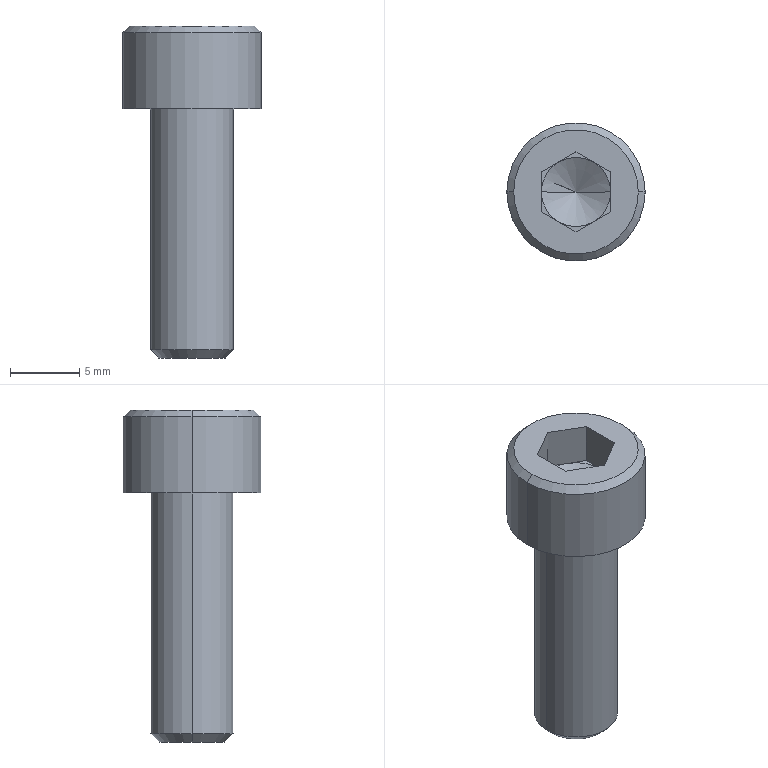Part | SolidWorks | features Chamfer 2, ICE 2, RevCut 1, Revolution 1 | 1 solid | 25 faces | box 10 x 10 x 24 mm | volume 898.677 mm3 | plane 15 | cone 6 | cylinder 4 | commonest cylinder face diameters 6 x2 10 x2
STEP:
#1=CARTESIAN_POINT('',(-2.387,0.,-18.));
#2=VERTEX_POINT('',#1);
#3=CARTESIAN_POINT('',(2.387,0.,-18.));
#4=VERTEX_POINT('',#3);
#5=CARTESIAN_POINT('',(0.,0.,-18.));
#6=DIRECTION('',(0.,0.,-1.));
#7=DIRECTION('',(-1.,0.,0.));
#8=AXIS2_PLACEMENT_3D('',#5,#6,#7);
#9=CIRCLE('',#8,2.387);
#10=EDGE_CURVE('',#2,#4,#9,.T.);
#11=ORIENTED_EDGE('',*,*,#10,.F.);
#12=CARTESIAN_POINT('',(-3.,0.,-17.387));
#13=VERTEX_POINT('',#12);
#14=CARTESIAN_POINT('',(-2.387,0.,-18.));
#15=DIRECTION('',(-0.7071,0.,0.7071));
#16=VECTOR('',#15,1000.);
#17=LINE('',#14,#16);
#18=EDGE_CURVE('',#2,#13,#17,.T.);
#19=ORIENTED_EDGE('',*,*,#18,.T.);
#20=CARTESIAN_POINT('',(3.,0.,-17.387));
#21=VERTEX_POINT('',#20);
#22=CARTESIAN_POINT('',(0.,0.,-17.387));
#23=DIRECTION('',(0.,0.,1.));
#24=DIRECTION('',(-1.,0.,0.));
#25=AXIS2_PLACEMENT_3D('',#22,#23,#24);
#26=CIRCLE('',#25,3.);
#27=EDGE_CURVE('',#21,#13,#26,.T.);
#28=ORIENTED_EDGE('',*,*,#27,.F.);
#29=CARTESIAN_POINT('',(2.387,0.,-18.));
#30=DIRECTION('',(0.7071,0.,0.7071));
#31=VECTOR('',#30,1000.);
#32=LINE('',#29,#31);
#33=EDGE_CURVE('',#4,#21,#32,.T.);
#34=ORIENTED_EDGE('',*,*,#33,.F.);
#35=EDGE_LOOP('',(#11,#19,#28,#34));
#36=FACE_OUTER_BOUND('',#35,.T.);
#37=CARTESIAN_POINT('',(0.,0.,-18.));
#38=DIRECTION('',(0.,0.,1.));
#39=DIRECTION('',(1.,0.,0.));
#40=AXIS2_PLACEMENT_3D('',#37,#38,#39);
#41=CONICAL_SURFACE('',#40,2.387,0.7854);
#42=ADVANCED_FACE('',(#36),#41,.T.);
#43=CARTESIAN_POINT('',(4.5,0.,6.));
#44=VERTEX_POINT('',#43);
#45=CARTESIAN_POINT('',(-4.5,0.,6.));
#46=VERTEX_POINT('',#45);
#47=CARTESIAN_POINT('',(0.,0.,6.));
#48=DIRECTION('',(0.,0.,1.));
#49=DIRECTION('',(1.,0.,0.));
#50=AXIS2_PLACEMENT_3D('',#47,#48,#49);
#51=CIRCLE('',#50,4.5);
#52=EDGE_CURVE('',#44,#46,#51,.T.);
#53=ORIENTED_EDGE('',*,*,#52,.F.);
#54=CARTESIAN_POINT('',(5.,0.,5.5));
#55=VERTEX_POINT('',#54);
#56=CARTESIAN_POINT('',(4.5,0.,6.));
#57=DIRECTION('',(0.7071,0.,-0.7071));
#58=VECTOR('',#57,1000.);
#59=LINE('',#56,#58);
#60=EDGE_CURVE('',#44,#55,#59,.T.);
#61=ORIENTED_EDGE('',*,*,#60,.T.);
#62=CARTESIAN_POINT('',(-5.,0.,5.5));
#63=VERTEX_POINT('',#62);
#64=CARTESIAN_POINT('',(0.,0.,5.5));
#65=DIRECTION('',(0.,0.,-1.));
#66=DIRECTION('',(1.,0.,0.));
#67=AXIS2_PLACEMENT_3D('',#64,#65,#66);
#68=CIRCLE('',#67,5.);
#69=EDGE_CURVE('',#63,#55,#68,.T.);
#70=ORIENTED_EDGE('',*,*,#69,.F.);
#71=CARTESIAN_POINT('',(-4.5,0.,6.));
#72=DIRECTION('',(-0.7071,0.,-0.7071));
#73=VECTOR('',#72,1000.);
#74=LINE('',#71,#73);
#75=EDGE_CURVE('',#46,#63,#74,.T.);
#76=ORIENTED_EDGE('',*,*,#75,.F.);
#77=EDGE_LOOP('',(#53,#61,#70,#76));
#78=FACE_OUTER_BOUND('',#77,.T.);
#79=CARTESIAN_POINT('',(0.,0.,6.));
#80=DIRECTION('',(0.,0.,-1.));
#81=DIRECTION('',(-1.,0.,0.));
#82=AXIS2_PLACEMENT_3D('',#79,#80,#81);
#83=CONICAL_SURFACE('',#82,4.5,0.7854);
#84=ADVANCED_FACE('',(#78),#83,.T.);
#85=CARTESIAN_POINT('',(0.,0.,1.557));
#86=VERTEX_POINT('',#85);
#87=CARTESIAN_POINT('',(2.5,0.,3.));
#88=VERTEX_POINT('',#87);
#89=CARTESIAN_POINT('',(0.,0.,1.557));
#90=DIRECTION('',(0.866,0.,0.5));
#91=VECTOR('',#90,1000.);
#92=LINE('',#89,#91);
#93=EDGE_CURVE('',#86,#88,#92,.T.);
#94=ORIENTED_EDGE('',*,*,#93,.F.);
#95=CARTESIAN_POINT('',(-2.5,0.,3.));
#96=VERTEX_POINT('',#95);
#97=CARTESIAN_POINT('',(0.,0.,1.557));
#98=DIRECTION('',(-0.866,0.,0.5));
#99=VECTOR('',#98,1000.);
#100=LINE('',#97,#99);
#101=EDGE_CURVE('',#86,#96,#100,.T.);
#102=ORIENTED_EDGE('',*,*,#101,.T.);
#103=CARTESIAN_POINT('',(-1.25,-2.165,3.));
#104=VERTEX_POINT('',#103);
#105=CARTESIAN_POINT('',(0.,0.,3.));
#106=DIRECTION('',(0.,0.,-1.));
#107=DIRECTION('',(-1.,0.,0.));
#108=AXIS2_PLACEMENT_3D('',#105,#106,#107);
#109=CIRCLE('',#108,2.5);
#110=EDGE_CURVE('',#104,#96,#109,.T.);
#111=ORIENTED_EDGE('',*,*,#110,.F.);
#112=CARTESIAN_POINT('',(1.25,-2.165,3.));
#113=VERTEX_POINT('',#112);
#114=CARTESIAN_POINT('',(0.,0.,3.));
#115=DIRECTION('',(0.,0.,-1.));
#116=DIRECTION('',(-1.,0.,0.));
#117=AXIS2_PLACEMENT_3D('',#114,#115,#116);
#118=CIRCLE('',#117,2.5);
#119=EDGE_CURVE('',#113,#104,#118,.T.);
#120=ORIENTED_EDGE('',*,*,#119,.F.);
#121=CARTESIAN_POINT('',(0.,0.,3.));
#122=DIRECTION('',(0.,0.,-1.));
#123=DIRECTION('',(-1.,0.,0.));
#124=AXIS2_PLACEMENT_3D('',#121,#122,#123);
#125=CIRCLE('',#124,2.5);
#126=EDGE_CURVE('',#88,#113,#125,.T.);
#127=ORIENTED_EDGE('',*,*,#126,.F.);
#128=EDGE_LOOP('',(#94,#102,#111,#120,#127));
#129=FACE_OUTER_BOUND('',#128,.T.);
#130=CARTESIAN_POINT('',(0.,0.,1001.557));
#131=DIRECTION('',(0.,0.,1.));
#132=DIRECTION('',(1.,0.,0.));
#133=AXIS2_PLACEMENT_3D('',#130,#131,#132);
#134=CONICAL_SURFACE('',#133,1732.051,1.047);
#135=ADVANCED_FACE('',(#129),#134,.F.);
#136=ORIENTED_EDGE('',*,*,#27,.T.);
#137=CARTESIAN_POINT('',(-3.,0.,0.));
#138=VERTEX_POINT('',#137);
#139=CARTESIAN_POINT('',(-3.,0.,-18.));
#140=DIRECTION('',(0.,0.,1.));
#141=VECTOR('',#140,1000.);
#142=LINE('',#139,#141);
#143=EDGE_CURVE('',#13,#138,#142,.T.);
#144=ORIENTED_EDGE('',*,*,#143,.T.);
#145=CARTESIAN_POINT('',(3.,0.,0.));
#146=VERTEX_POINT('',#145);
#147=CARTESIAN_POINT('',(0.,0.,0.));
#148=DIRECTION('',(0.,0.,-1.));
#149=DIRECTION('',(-1.,0.,0.));
#150=AXIS2_PLACEMENT_3D('',#147,#148,#149);
#151=CIRCLE('',#150,3.);
#152=EDGE_CURVE('',#138,#146,#151,.T.);
#153=ORIENTED_EDGE('',*,*,#152,.T.);
#154=CARTESIAN_POINT('',(3.,0.,-18.));
#155=DIRECTION('',(0.,0.,1.));
#156=VECTOR('',#155,1000.);
#157=LINE('',#154,#156);
#158=EDGE_CURVE('',#21,#146,#157,.T.);
#159=ORIENTED_EDGE('',*,*,#158,.F.);
#160=EDGE_LOOP('',(#136,#144,#153,#159));
#161=FACE_OUTER_BOUND('',#160,.T.);
#162=CARTESIAN_POINT('',(0.,0.,-18.));
#163=DIRECTION('',(0.,0.,1.));
#164=DIRECTION('',(1.,0.,0.));
#165=AXIS2_PLACEMENT_3D('',#162,#163,#164);
#166=CYLINDRICAL_SURFACE('',#165,3.);
#167=ADVANCED_FACE('',(#161),#166,.T.);
#168=CARTESIAN_POINT('',(5.,0.,0.));
#169=VERTEX_POINT('',#168);
#170=CARTESIAN_POINT('',(-5.,0.,0.));
#171=VERTEX_POINT('',#170);
#172=CARTESIAN_POINT('',(0.,0.,0.));
#173=DIRECTION('',(0.,0.,1.));
#174=DIRECTION('',(1.,0.,0.));
#175=AXIS2_PLACEMENT_3D('',#172,#173,#174);
#176=CIRCLE('',#175,5.);
#177=EDGE_CURVE('',#169,#171,#176,.T.);
#178=ORIENTED_EDGE('',*,*,#177,.T.);
#179=CARTESIAN_POINT('',(-5.,0.,0.));
#180=DIRECTION('',(0.,0.,1.));
#181=VECTOR('',#180,1000.);
#182=LINE('',#179,#181);
#183=EDGE_CURVE('',#171,#63,#182,.T.);
#184=ORIENTED_EDGE('',*,*,#183,.T.);
#185=ORIENTED_EDGE('',*,*,#69,.T.);
#186=CARTESIAN_POINT('',(5.,0.,0.));
#187=DIRECTION('',(0.,0.,1.));
#188=VECTOR('',#187,1000.);
#189=LINE('',#186,#188);
#190=EDGE_CURVE('',#169,#55,#189,.T.);
#191=ORIENTED_EDGE('',*,*,#190,.F.);
#192=EDGE_LOOP('',(#178,#184,#185,#191));
#193=FACE_OUTER_BOUND('',#192,.T.);
#194=CARTESIAN_POINT('',(0.,0.,0.));
#195=DIRECTION('',(0.,0.,1.));
#196=DIRECTION('',(1.,0.,0.));
#197=AXIS2_PLACEMENT_3D('',#194,#195,#196);
#198=CYLINDRICAL_SURFACE('',#197,5.);
#199=ADVANCED_FACE('',(#193),#198,.T.);
#200=CARTESIAN_POINT('',(-2.5,1.443,3.));
#201=VERTEX_POINT('',#200);
#202=CARTESIAN_POINT('',(-2.5,1.443,3.));
#203=DIRECTION('',(0.,-1.,0.));
#204=VECTOR('',#203,1000.);
#205=LINE('',#202,#204);
#206=EDGE_CURVE('',#201,#96,#205,.T.);
#207=ORIENTED_EDGE('',*,*,#206,.T.);
#208=CARTESIAN_POINT('',(-1.25,2.165,3.));
#209=VERTEX_POINT('',#208);
#210=CARTESIAN_POINT('',(0.,0.,3.));
#211=DIRECTION('',(0.,0.,-1.));
#212=DIRECTION('',(-1.,0.,0.));
#213=AXIS2_PLACEMENT_3D('',#210,#211,#212);
#214=CIRCLE('',#213,2.5);
#215=EDGE_CURVE('',#96,#209,#214,.T.);
#216=ORIENTED_EDGE('',*,*,#215,.T.);
#217=CARTESIAN_POINT('',(0.,2.887,3.));
#218=DIRECTION('',(-0.866,-0.5,0.));
#219=VECTOR('',#218,1000.);
#220=LINE('',#217,#219);
#221=EDGE_CURVE('',#209,#201,#220,.T.);
#222=ORIENTED_EDGE('',*,*,#221,.T.);
#223=EDGE_LOOP('',(#207,#216,#222));
#224=FACE_OUTER_BOUND('',#223,.T.);
#225=CARTESIAN_POINT('',(0.,0.,3.));
#226=DIRECTION('',(0.,0.,1.));
#227=DIRECTION('',(1.,0.,0.));
#228=AXIS2_PLACEMENT_3D('',#225,#226,#227);
#229=PLANE('',#228);
#230=ADVANCED_FACE('',(#224),#229,.T.);
#231=CARTESIAN_POINT('',(0.,2.887,3.));
#232=VERTEX_POINT('',#231);
#233=CARTESIAN_POINT('',(0.,2.887,3.));
#234=DIRECTION('',(-0.866,-0.5,0.));
#235=VECTOR('',#234,1000.);
#236=LINE('',#233,#235);
#237=EDGE_CURVE('',#232,#209,#236,.T.);
#238=ORIENTED_EDGE('',*,*,#237,.T.);
#239=CARTESIAN_POINT('',(1.25,2.165,3.));
#240=VERTEX_POINT('',#239);
#241=CARTESIAN_POINT('',(0.,0.,3.));
#242=DIRECTION('',(0.,0.,-1.));
#243=DIRECTION('',(-1.,0.,0.));
#244=AXIS2_PLACEMENT_3D('',#241,#242,#243);
#245=CIRCLE('',#244,2.5);
#246=EDGE_CURVE('',#209,#240,#245,.T.);
#247=ORIENTED_EDGE('',*,*,#246,.T.);
#248=CARTESIAN_POINT('',(2.5,1.443,3.));
#249=DIRECTION('',(-0.866,0.5,0.));
#250=VECTOR('',#249,1000.);
#251=LINE('',#248,#250);
#252=EDGE_CURVE('',#240,#232,#251,.T.);
#253=ORIENTED_EDGE('',*,*,#252,.T.);
#254=EDGE_LOOP('',(#238,#247,#253));
#255=FACE_OUTER_BOUND('',#254,.T.);
#256=CARTESIAN_POINT('',(0.,0.,3.));
#257=DIRECTION('',(0.,0.,1.));
#258=DIRECTION('',(1.,0.,0.));
#259=AXIS2_PLACEMENT_3D('',#256,#257,#258);
#260=PLANE('',#259);
#261=ADVANCED_FACE('',(#255),#260,.T.);
#262=CARTESIAN_POINT('',(2.5,1.443,3.));
#263=VERTEX_POINT('',#262);
#264=CARTESIAN_POINT('',(2.5,1.443,3.));
#265=DIRECTION('',(-0.866,0.5,0.));
#266=VECTOR('',#265,1000.);
#267=LINE('',#264,#266);
#268=EDGE_CURVE('',#263,#240,#267,.T.);
#269=ORIENTED_EDGE('',*,*,#268,.T.);
#270=CARTESIAN_POINT('',(0.,0.,3.));
#271=DIRECTION('',(0.,0.,-1.));
#272=DIRECTION('',(-1.,0.,0.));
#273=AXIS2_PLACEMENT_3D('',#270,#271,#272);
#274=CIRCLE('',#273,2.5);
#275=EDGE_CURVE('',#240,#88,#274,.T.);
#276=ORIENTED_EDGE('',*,*,#275,.T.);
#277=CARTESIAN_POINT('',(2.5,-1.443,3.));
#278=DIRECTION('',(0.,1.,0.));
#279=VECTOR('',#278,1000.);
#280=LINE('',#277,#279);
#281=EDGE_CURVE('',#88,#263,#280,.T.);
#282=ORIENTED_EDGE('',*,*,#281,.T.);
#283=EDGE_LOOP('',(#269,#276,#282));
#284=FACE_OUTER_BOUND('',#283,.T.);
#285=CARTESIAN_POINT('',(0.,0.,3.));
#286=DIRECTION('',(0.,0.,1.));
#287=DIRECTION('',(1.,0.,0.));
#288=AXIS2_PLACEMENT_3D('',#285,#286,#287);
#289=PLANE('',#288);
#290=ADVANCED_FACE('',(#284),#289,.T.);
#291=CARTESIAN_POINT('',(2.5,-1.443,3.));
#292=VERTEX_POINT('',#291);
#293=CARTESIAN_POINT('',(2.5,-1.443,3.));
#294=DIRECTION('',(0.,1.,0.));
#295=VECTOR('',#294,1000.);
#296=LINE('',#293,#295);
#297=EDGE_CURVE('',#292,#88,#296,.T.);
#298=ORIENTED_EDGE('',*,*,#297,.T.);
#299=ORIENTED_EDGE('',*,*,#126,.T.);
#300=CARTESIAN_POINT('',(0.,-2.887,3.));
#301=DIRECTION('',(0.866,0.5,0.));
#302=VECTOR('',#301,1000.);
#303=LINE('',#300,#302);
#304=EDGE_CURVE('',#113,#292,#303,.T.);
#305=ORIENTED_EDGE('',*,*,#304,.T.);
#306=EDGE_LOOP('',(#298,#299,#305));
#307=FACE_OUTER_BOUND('',#306,.T.);
#308=CARTESIAN_POINT('',(0.,0.,3.));
#309=DIRECTION('',(0.,0.,1.));
#310=DIRECTION('',(1.,0.,0.));
#311=AXIS2_PLACEMENT_3D('',#308,#309,#310);
#312=PLANE('',#311);
#313=ADVANCED_FACE('',(#307),#312,.T.);
#314=CARTESIAN_POINT('',(0.,-2.887,3.));
#315=VERTEX_POINT('',#314);
#316=CARTESIAN_POINT('',(0.,-2.887,3.));
#317=DIRECTION('',(0.866,0.5,0.));
#318=VECTOR('',#317,1000.);
#319=LINE('',#316,#318);
#320=EDGE_CURVE('',#315,#113,#319,.T.);
#321=ORIENTED_EDGE('',*,*,#320,.T.);
#322=ORIENTED_EDGE('',*,*,#119,.T.);
#323=CARTESIAN_POINT('',(-2.5,-1.443,3.));
#324=DIRECTION('',(0.866,-0.5,0.));
#325=VECTOR('',#324,1000.);
#326=LINE('',#323,#325);
#327=EDGE_CURVE('',#104,#315,#326,.T.);
#328=ORIENTED_EDGE('',*,*,#327,.T.);
#329=EDGE_LOOP('',(#321,#322,#328));
#330=FACE_OUTER_BOUND('',#329,.T.);
#331=CARTESIAN_POINT('',(0.,0.,3.));
#332=DIRECTION('',(0.,0.,1.));
#333=DIRECTION('',(1.,0.,0.));
#334=AXIS2_PLACEMENT_3D('',#331,#332,#333);
#335=PLANE('',#334);
#336=ADVANCED_FACE('',(#330),#335,.T.);
#337=CARTESIAN_POINT('',(-2.5,-1.443,3.));
#338=VERTEX_POINT('',#337);
#339=CARTESIAN_POINT('',(-2.5,-1.443,3.));
#340=DIRECTION('',(0.866,-0.5,0.));
#341=VECTOR('',#340,1000.);
#342=LINE('',#339,#341);
#343=EDGE_CURVE('',#338,#104,#342,.T.);
#344=ORIENTED_EDGE('',*,*,#343,.T.);
#345=ORIENTED_EDGE('',*,*,#110,.T.);
#346=CARTESIAN_POINT('',(-2.5,1.443,3.));
#347=DIRECTION('',(0.,-1.,0.));
#348=VECTOR('',#347,1000.);
#349=LINE('',#346,#348);
#350=EDGE_CURVE('',#96,#338,#349,.T.);
#351=ORIENTED_EDGE('',*,*,#350,.T.);
#352=EDGE_LOOP('',(#344,#345,#351));
#353=FACE_OUTER_BOUND('',#352,.T.);
#354=CARTESIAN_POINT('',(0.,0.,3.));
#355=DIRECTION('',(0.,0.,1.));
#356=DIRECTION('',(1.,0.,0.));
#357=AXIS2_PLACEMENT_3D('',#354,#355,#356);
#358=PLANE('',#357);
#359=ADVANCED_FACE('',(#353),#358,.T.);
#360=ORIENTED_EDGE('',*,*,#177,.F.);
#361=CARTESIAN_POINT('',(0.,0.,0.));
#362=DIRECTION('',(0.,0.,1.));
#363=DIRECTION('',(1.,0.,0.));
#364=AXIS2_PLACEMENT_3D('',#361,#362,#363);
#365=CIRCLE('',#364,5.);
#366=EDGE_CURVE('',#171,#169,#365,.T.);
#367=ORIENTED_EDGE('',*,*,#366,.F.);
#368=EDGE_LOOP('',(#360,#367));
#369=FACE_OUTER_BOUND('',#368,.T.);
#370=CARTESIAN_POINT('',(0.,0.,0.));
#371=DIRECTION('',(0.,0.,-1.));
#372=DIRECTION('',(-1.,0.,0.));
#373=AXIS2_PLACEMENT_3D('',#370,#371,#372);
#374=CIRCLE('',#373,3.);
#375=EDGE_CURVE('',#146,#138,#374,.T.);
#376=ORIENTED_EDGE('',*,*,#375,.F.);
#377=ORIENTED_EDGE('',*,*,#152,.F.);
#378=EDGE_LOOP('',(#376,#377));
#379=FACE_BOUND('',#378,.T.);
#380=CARTESIAN_POINT('',(5.,0.,0.));
#381=DIRECTION('',(0.,0.,-1.));
#382=DIRECTION('',(-1.,0.,0.));
#383=AXIS2_PLACEMENT_3D('',#380,#381,#382);
#384=PLANE('',#383);
#385=ADVANCED_FACE('',(#369,#379),#384,.T.);
#386=ORIENTED_EDGE('',*,*,#183,.F.);
#387=ORIENTED_EDGE('',*,*,#366,.T.);
#388=ORIENTED_EDGE('',*,*,#190,.T.);
#389=CARTESIAN_POINT('',(0.,0.,5.5));
#390=DIRECTION('',(0.,0.,-1.));
#391=DIRECTION('',(1.,0.,0.));
#392=AXIS2_PLACEMENT_3D('',#389,#390,#391);
#393=CIRCLE('',#392,5.);
#394=EDGE_CURVE('',#55,#63,#393,.T.);
#395=ORIENTED_EDGE('',*,*,#394,.T.);
#396=EDGE_LOOP('',(#386,#387,#388,#395));
#397=FACE_OUTER_BOUND('',#396,.T.);
#398=CARTESIAN_POINT('',(0.,0.,0.));
#399=DIRECTION('',(0.,0.,1.));
#400=DIRECTION('',(1.,0.,0.));
#401=AXIS2_PLACEMENT_3D('',#398,#399,#400);
#402=CYLINDRICAL_SURFACE('',#401,5.);
#403=ADVANCED_FACE('',(#397),#402,.T.);
#404=CARTESIAN_POINT('',(0.,0.,6.));
#405=DIRECTION('',(0.,0.,1.));
#406=DIRECTION('',(1.,0.,0.));
#407=AXIS2_PLACEMENT_3D('',#404,#405,#406);
#408=CIRCLE('',#407,4.5);
#409=EDGE_CURVE('',#46,#44,#408,.T.);
#410=ORIENTED_EDGE('',*,*,#409,.T.);
#411=ORIENTED_EDGE('',*,*,#52,.T.);
#412=EDGE_LOOP('',(#410,#411));
#413=FACE_OUTER_BOUND('',#412,.T.);
#414=CARTESIAN_POINT('',(2.5,-1.443,6.));
#415=VERTEX_POINT('',#414);
#416=CARTESIAN_POINT('',(2.5,1.443,6.));
#417=VERTEX_POINT('',#416);
#418=CARTESIAN_POINT('',(2.5,-1.443,6.));
#419=DIRECTION('',(0.,1.,0.));
#420=VECTOR('',#419,1000.);
#421=LINE('',#418,#420);
#422=EDGE_CURVE('',#415,#417,#421,.T.);
#423=ORIENTED_EDGE('',*,*,#422,.F.);
#424=CARTESIAN_POINT('',(0.,-2.887,6.));
#425=VERTEX_POINT('',#424);
#426=CARTESIAN_POINT('',(0.,-2.887,6.));
#427=DIRECTION('',(0.866,0.5,0.));
#428=VECTOR('',#427,1000.);
#429=LINE('',#426,#428);
#430=EDGE_CURVE('',#425,#415,#429,.T.);
#431=ORIENTED_EDGE('',*,*,#430,.F.);
#432=CARTESIAN_POINT('',(-2.5,-1.443,6.));
#433=VERTEX_POINT('',#432);
#434=CARTESIAN_POINT('',(-2.5,-1.443,6.));
#435=DIRECTION('',(0.866,-0.5,0.));
#436=VECTOR('',#435,1000.);
#437=LINE('',#434,#436);
#438=EDGE_CURVE('',#433,#425,#437,.T.);
#439=ORIENTED_EDGE('',*,*,#438,.F.);
#440=CARTESIAN_POINT('',(-2.5,1.443,6.));
#441=VERTEX_POINT('',#440);
#442=CARTESIAN_POINT('',(-2.5,1.443,6.));
#443=DIRECTION('',(0.,-1.,0.));
#444=VECTOR('',#443,1000.);
#445=LINE('',#442,#444);
#446=EDGE_CURVE('',#441,#433,#445,.T.);
#447=ORIENTED_EDGE('',*,*,#446,.F.);
#448=CARTESIAN_POINT('',(0.,2.887,6.));
#449=VERTEX_POINT('',#448);
#450=CARTESIAN_POINT('',(0.,2.887,6.));
#451=DIRECTION('',(-0.866,-0.5,0.));
#452=VECTOR('',#451,1000.);
#453=LINE('',#450,#452);
#454=EDGE_CURVE('',#449,#441,#453,.T.);
#455=ORIENTED_EDGE('',*,*,#454,.F.);
#456=CARTESIAN_POINT('',(2.5,1.443,6.));
#457=DIRECTION('',(-0.866,0.5,0.));
#458=VECTOR('',#457,1000.);
#459=LINE('',#456,#458);
#460=EDGE_CURVE('',#417,#449,#459,.T.);
#461=ORIENTED_EDGE('',*,*,#460,.F.);
#462=EDGE_LOOP('',(#423,#431,#439,#447,#455,#461));
#463=FACE_BOUND('',#462,.T.);
#464=CARTESIAN_POINT('',(0.,0.,6.));
#465=DIRECTION('',(0.,0.,1.));
#466=DIRECTION('',(1.,0.,0.));
#467=AXIS2_PLACEMENT_3D('',#464,#465,#466);
#468=PLANE('',#467);
#469=ADVANCED_FACE('',(#413,#463),#468,.T.);
#470=ORIENTED_EDGE('',*,*,#143,.F.);
#471=CARTESIAN_POINT('',(0.,0.,-17.387));
#472=DIRECTION('',(0.,0.,1.));
#473=DIRECTION('',(-1.,0.,0.));
#474=AXIS2_PLACEMENT_3D('',#471,#472,#473);
#475=CIRCLE('',#474,3.);
#476=EDGE_CURVE('',#13,#21,#475,.T.);
#477=ORIENTED_EDGE('',*,*,#476,.T.);
#478=ORIENTED_EDGE('',*,*,#158,.T.);
#479=ORIENTED_EDGE('',*,*,#375,.T.);
#480=EDGE_LOOP('',(#470,#477,#478,#479));
#481=FACE_OUTER_BOUND('',#480,.T.);
#482=CARTESIAN_POINT('',(0.,0.,-18.));
#483=DIRECTION('',(0.,0.,1.));
#484=DIRECTION('',(1.,0.,0.));
#485=AXIS2_PLACEMENT_3D('',#482,#483,#484);
#486=CYLINDRICAL_SURFACE('',#485,3.);
#487=ADVANCED_FACE('',(#481),#486,.T.);
#488=CARTESIAN_POINT('',(0.,0.,-18.));
#489=DIRECTION('',(0.,0.,-1.));
#490=DIRECTION('',(-1.,0.,0.));
#491=AXIS2_PLACEMENT_3D('',#488,#489,#490);
#492=CIRCLE('',#491,2.387);
#493=EDGE_CURVE('',#4,#2,#492,.T.);
#494=ORIENTED_EDGE('',*,*,#493,.T.);
#495=ORIENTED_EDGE('',*,*,#10,.T.);
#496=EDGE_LOOP('',(#494,#495));
#497=FACE_OUTER_BOUND('',#496,.T.);
#498=CARTESIAN_POINT('',(0.,0.,-18.));
#499=DIRECTION('',(0.,0.,-1.));
#500=DIRECTION('',(-1.,0.,0.));
#501=AXIS2_PLACEMENT_3D('',#498,#499,#500);
#502=PLANE('',#501);
#503=ADVANCED_FACE('',(#497),#502,.T.);
#504=ORIENTED_EDGE('',*,*,#422,.T.);
#505=CARTESIAN_POINT('',(2.5,1.443,3.));
#506=DIRECTION('',(0.,0.,1.));
#507=VECTOR('',#506,1000.);
#508=LINE('',#505,#507);
#509=EDGE_CURVE('',#263,#417,#508,.T.);
#510=ORIENTED_EDGE('',*,*,#509,.F.);
#511=ORIENTED_EDGE('',*,*,#281,.F.);
#512=ORIENTED_EDGE('',*,*,#297,.F.);
#513=CARTESIAN_POINT('',(2.5,-1.443,3.));
#514=DIRECTION('',(0.,0.,1.));
#515=VECTOR('',#514,1000.);
#516=LINE('',#513,#515);
#517=EDGE_CURVE('',#292,#415,#516,.T.);
#518=ORIENTED_EDGE('',*,*,#517,.T.);
#519=EDGE_LOOP('',(#504,#510,#511,#512,#518));
#520=FACE_OUTER_BOUND('',#519,.T.);
#521=CARTESIAN_POINT('',(2.5,-1.443,3.));
#522=DIRECTION('',(1.,0.,0.));
#523=DIRECTION('',(0.,1.,0.));
#524=AXIS2_PLACEMENT_3D('',#521,#522,#523);
#525=PLANE('',#524);
#526=ADVANCED_FACE('',(#520),#525,.F.);
#527=ORIENTED_EDGE('',*,*,#430,.T.);
#528=ORIENTED_EDGE('',*,*,#517,.F.);
#529=ORIENTED_EDGE('',*,*,#304,.F.);
#530=ORIENTED_EDGE('',*,*,#320,.F.);
#531=CARTESIAN_POINT('',(0.,-2.887,3.));
#532=DIRECTION('',(0.,0.,1.));
#533=VECTOR('',#532,1000.);
#534=LINE('',#531,#533);
#535=EDGE_CURVE('',#315,#425,#534,.T.);
#536=ORIENTED_EDGE('',*,*,#535,.T.);
#537=EDGE_LOOP('',(#527,#528,#529,#530,#536));
#538=FACE_OUTER_BOUND('',#537,.T.);
#539=CARTESIAN_POINT('',(0.,-2.887,3.));
#540=DIRECTION('',(0.5,-0.866,0.));
#541=DIRECTION('',(0.866,0.5,0.));
#542=AXIS2_PLACEMENT_3D('',#539,#540,#541);
#543=PLANE('',#542);
#544=ADVANCED_FACE('',(#538),#543,.F.);
#545=ORIENTED_EDGE('',*,*,#438,.T.);
#546=ORIENTED_EDGE('',*,*,#535,.F.);
#547=ORIENTED_EDGE('',*,*,#327,.F.);
#548=ORIENTED_EDGE('',*,*,#343,.F.);
#549=CARTESIAN_POINT('',(-2.5,-1.443,3.));
#550=DIRECTION('',(0.,0.,1.));
#551=VECTOR('',#550,1000.);
#552=LINE('',#549,#551);
#553=EDGE_CURVE('',#338,#433,#552,.T.);
#554=ORIENTED_EDGE('',*,*,#553,.T.);
#555=EDGE_LOOP('',(#545,#546,#547,#548,#554));
#556=FACE_OUTER_BOUND('',#555,.T.);
#557=CARTESIAN_POINT('',(-2.5,-1.443,3.));
#558=DIRECTION('',(-0.5,-0.866,0.));
#559=DIRECTION('',(0.866,-0.5,0.));
#560=AXIS2_PLACEMENT_3D('',#557,#558,#559);
#561=PLANE('',#560);
#562=ADVANCED_FACE('',(#556),#561,.F.);
#563=ORIENTED_EDGE('',*,*,#446,.T.);
#564=ORIENTED_EDGE('',*,*,#553,.F.);
#565=ORIENTED_EDGE('',*,*,#350,.F.);
#566=ORIENTED_EDGE('',*,*,#206,.F.);
#567=CARTESIAN_POINT('',(-2.5,1.443,3.));
#568=DIRECTION('',(0.,0.,1.));
#569=VECTOR('',#568,1000.);
#570=LINE('',#567,#569);
#571=EDGE_CURVE('',#201,#441,#570,.T.);
#572=ORIENTED_EDGE('',*,*,#571,.T.);
#573=EDGE_LOOP('',(#563,#564,#565,#566,#572));
#574=FACE_OUTER_BOUND('',#573,.T.);
#575=CARTESIAN_POINT('',(-2.5,1.443,3.));
#576=DIRECTION('',(-1.,0.,0.));
#577=DIRECTION('',(0.,-1.,0.));
#578=AXIS2_PLACEMENT_3D('',#575,#576,#577);
#579=PLANE('',#578);
#580=ADVANCED_FACE('',(#574),#579,.F.);
#581=ORIENTED_EDGE('',*,*,#454,.T.);
#582=ORIENTED_EDGE('',*,*,#571,.F.);
#583=ORIENTED_EDGE('',*,*,#221,.F.);
#584=ORIENTED_EDGE('',*,*,#237,.F.);
#585=CARTESIAN_POINT('',(0.,2.887,3.));
#586=DIRECTION('',(0.,0.,1.));
#587=VECTOR('',#586,1000.);
#588=LINE('',#585,#587);
#589=EDGE_CURVE('',#232,#449,#588,.T.);
#590=ORIENTED_EDGE('',*,*,#589,.T.);
#591=EDGE_LOOP('',(#581,#582,#583,#584,#590));
#592=FACE_OUTER_BOUND('',#591,.T.);
#593=CARTESIAN_POINT('',(0.,2.887,3.));
#594=DIRECTION('',(-0.5,0.866,0.));
#595=DIRECTION('',(-0.866,-0.5,0.));
#596=AXIS2_PLACEMENT_3D('',#593,#594,#595);
#597=PLANE('',#596);
#598=ADVANCED_FACE('',(#592),#597,.F.);
#599=ORIENTED_EDGE('',*,*,#460,.T.);
#600=ORIENTED_EDGE('',*,*,#589,.F.);
#601=ORIENTED_EDGE('',*,*,#252,.F.);
#602=ORIENTED_EDGE('',*,*,#268,.F.);
#603=ORIENTED_EDGE('',*,*,#509,.T.);
#604=EDGE_LOOP('',(#599,#600,#601,#602,#603));
#605=FACE_OUTER_BOUND('',#604,.T.);
#606=CARTESIAN_POINT('',(2.5,1.443,3.));
#607=DIRECTION('',(0.5,0.866,0.));
#608=DIRECTION('',(-0.866,0.5,0.));
#609=AXIS2_PLACEMENT_3D('',#606,#607,#608);
#610=PLANE('',#609);
#611=ADVANCED_FACE('',(#605),#610,.F.);
#612=ORIENTED_EDGE('',*,*,#101,.F.);
#613=ORIENTED_EDGE('',*,*,#93,.T.);
#614=ORIENTED_EDGE('',*,*,#275,.F.);
#615=ORIENTED_EDGE('',*,*,#246,.F.);
#616=ORIENTED_EDGE('',*,*,#215,.F.);
#617=EDGE_LOOP('',(#612,#613,#614,#615,#616));
#618=FACE_OUTER_BOUND('',#617,.T.);
#619=CARTESIAN_POINT('',(0.,0.,1001.557));
#620=DIRECTION('',(0.,0.,1.));
#621=DIRECTION('',(1.,0.,0.));
#622=AXIS2_PLACEMENT_3D('',#619,#620,#621);
#623=CONICAL_SURFACE('',#622,1732.051,1.047);
#624=ADVANCED_FACE('',(#618),#623,.F.);
#625=ORIENTED_EDGE('',*,*,#60,.F.);
#626=ORIENTED_EDGE('',*,*,#409,.F.);
#627=ORIENTED_EDGE('',*,*,#75,.T.);
#628=ORIENTED_EDGE('',*,*,#394,.F.);
#629=EDGE_LOOP('',(#625,#626,#627,#628));
#630=FACE_OUTER_BOUND('',#629,.T.);
#631=CARTESIAN_POINT('',(0.,0.,6.));
#632=DIRECTION('',(0.,0.,-1.));
#633=DIRECTION('',(-1.,0.,0.));
#634=AXIS2_PLACEMENT_3D('',#631,#632,#633);
#635=CONICAL_SURFACE('',#634,4.5,0.7854);
#636=ADVANCED_FACE('',(#630),#635,.T.);
#637=ORIENTED_EDGE('',*,*,#18,.F.);
#638=ORIENTED_EDGE('',*,*,#493,.F.);
#639=ORIENTED_EDGE('',*,*,#33,.T.);
#640=ORIENTED_EDGE('',*,*,#476,.F.);
#641=EDGE_LOOP('',(#637,#638,#639,#640));
#642=FACE_OUTER_BOUND('',#641,.T.);
#643=CARTESIAN_POINT('',(0.,0.,-18.));
#644=DIRECTION('',(0.,0.,1.));
#645=DIRECTION('',(1.,0.,0.));
#646=AXIS2_PLACEMENT_3D('',#643,#644,#645);
#647=CONICAL_SURFACE('',#646,2.387,0.7854);
#648=ADVANCED_FACE('',(#642),#647,.T.);
#649=CLOSED_SHELL('',(#42,#84,#135,#167,#199,#230,#261,#290,#313,#336,#359,#385,#403,#469,#487,#503,#526,#544,#562,#580,#598,#611,#624,#636,#648));
#650=MANIFOLD_SOLID_BREP('',#649);
#651=CARTESIAN_POINT('',(0.,0.,0.));
#652=DIRECTION('',(0.,0.,1.));
#653=DIRECTION('',(1.,0.,0.));
#654=AXIS2_PLACEMENT_3D('',#651,#652,#653);
#655=(LENGTH_UNIT()NAMED_UNIT(*)SI_UNIT(.MILLI.,.METRE.));
#656=UNCERTAINTY_MEASURE_WITH_UNIT(LENGTH_MEASURE(0.00001),#655,'','');
#657=(NAMED_UNIT(*)PLANE_ANGLE_UNIT()SI_UNIT($,.RADIAN.));
#658=(NAMED_UNIT(*)SI_UNIT($,.STERADIAN.)SOLID_ANGLE_UNIT());
#659=(GEOMETRIC_REPRESENTATION_CONTEXT(3)GLOBAL_UNCERTAINTY_ASSIGNED_CONTEXT((#656))GLOBAL_UNIT_ASSIGNED_CONTEXT((#655,#657,#658))REPRESENTATION_CONTEXT('',''));
#660=ADVANCED_BREP_SHAPE_REPRESENTATION('',(#650,#654),#659);